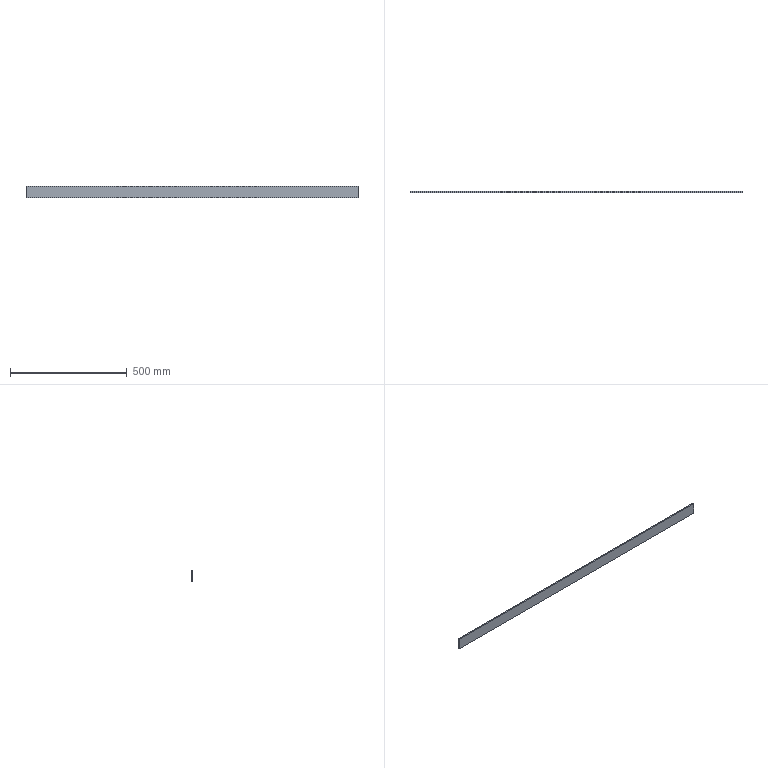Part | STEP file | Gripper baffle | 1 solid | 6 faces | box 1420 x 5 x 50 mm | volume 355000 mm3 | plane 6
STEP:
#1=CARTESIAN_POINT('',(710.,0.,25.));
#2=VERTEX_POINT('',#1);
#3=CARTESIAN_POINT('',(710.,0.,-25.));
#4=VERTEX_POINT('',#3);
#5=CARTESIAN_POINT('',(710.,0.,-25.));
#6=DIRECTION('',(0.,0.,-1.));
#7=VECTOR('',#6,1000.);
#8=LINE('',#5,#7);
#9=EDGE_CURVE('',#2,#4,#8,.T.);
#10=ORIENTED_EDGE('',*,*,#9,.T.);
#11=CARTESIAN_POINT('',(710.,5.,-25.));
#12=VERTEX_POINT('',#11);
#13=CARTESIAN_POINT('',(710.,5.,-25.));
#14=DIRECTION('',(0.,-1.,0.));
#15=VECTOR('',#14,1000.);
#16=LINE('',#13,#15);
#17=EDGE_CURVE('',#12,#4,#16,.T.);
#18=ORIENTED_EDGE('',*,*,#17,.F.);
#19=CARTESIAN_POINT('',(710.,5.,25.));
#20=VERTEX_POINT('',#19);
#21=CARTESIAN_POINT('',(710.,5.,-25.));
#22=DIRECTION('',(0.,0.,-1.));
#23=VECTOR('',#22,1000.);
#24=LINE('',#21,#23);
#25=EDGE_CURVE('',#20,#12,#24,.T.);
#26=ORIENTED_EDGE('',*,*,#25,.F.);
#27=CARTESIAN_POINT('',(710.,5.,25.));
#28=DIRECTION('',(0.,-1.,0.));
#29=VECTOR('',#28,1000.);
#30=LINE('',#27,#29);
#31=EDGE_CURVE('',#20,#2,#30,.T.);
#32=ORIENTED_EDGE('',*,*,#31,.T.);
#33=EDGE_LOOP('',(#10,#18,#26,#32));
#34=FACE_OUTER_BOUND('',#33,.T.);
#35=CARTESIAN_POINT('',(710.,5.,-25.));
#36=DIRECTION('',(-1.,0.,0.));
#37=DIRECTION('',(0.,0.,1.));
#38=AXIS2_PLACEMENT_3D('',#35,#36,#37);
#39=PLANE('',#38);
#40=ADVANCED_FACE('',(#34),#39,.F.);
#41=CARTESIAN_POINT('',(-710.,0.,-25.));
#42=VERTEX_POINT('',#41);
#43=CARTESIAN_POINT('',(-710.,0.,-25.));
#44=DIRECTION('',(-1.,0.,0.));
#45=VECTOR('',#44,1000.);
#46=LINE('',#43,#45);
#47=EDGE_CURVE('',#4,#42,#46,.T.);
#48=ORIENTED_EDGE('',*,*,#47,.T.);
#49=CARTESIAN_POINT('',(-710.,5.,-25.));
#50=VERTEX_POINT('',#49);
#51=CARTESIAN_POINT('',(-710.,5.,-25.));
#52=DIRECTION('',(0.,-1.,0.));
#53=VECTOR('',#52,1000.);
#54=LINE('',#51,#53);
#55=EDGE_CURVE('',#50,#42,#54,.T.);
#56=ORIENTED_EDGE('',*,*,#55,.F.);
#57=CARTESIAN_POINT('',(-710.,5.,-25.));
#58=DIRECTION('',(-1.,0.,0.));
#59=VECTOR('',#58,1000.);
#60=LINE('',#57,#59);
#61=EDGE_CURVE('',#12,#50,#60,.T.);
#62=ORIENTED_EDGE('',*,*,#61,.F.);
#63=ORIENTED_EDGE('',*,*,#17,.T.);
#64=EDGE_LOOP('',(#48,#56,#62,#63));
#65=FACE_OUTER_BOUND('',#64,.T.);
#66=CARTESIAN_POINT('',(-710.,5.,-25.));
#67=DIRECTION('',(0.,0.,1.));
#68=DIRECTION('',(1.,0.,0.));
#69=AXIS2_PLACEMENT_3D('',#66,#67,#68);
#70=PLANE('',#69);
#71=ADVANCED_FACE('',(#65),#70,.F.);
#72=CARTESIAN_POINT('',(-710.,0.,25.));
#73=VERTEX_POINT('',#72);
#74=CARTESIAN_POINT('',(-710.,0.,-25.));
#75=DIRECTION('',(0.,0.,1.));
#76=VECTOR('',#75,1000.);
#77=LINE('',#74,#76);
#78=EDGE_CURVE('',#42,#73,#77,.T.);
#79=ORIENTED_EDGE('',*,*,#78,.T.);
#80=CARTESIAN_POINT('',(-710.,5.,25.));
#81=VERTEX_POINT('',#80);
#82=CARTESIAN_POINT('',(-710.,5.,25.));
#83=DIRECTION('',(0.,-1.,0.));
#84=VECTOR('',#83,1000.);
#85=LINE('',#82,#84);
#86=EDGE_CURVE('',#81,#73,#85,.T.);
#87=ORIENTED_EDGE('',*,*,#86,.F.);
#88=CARTESIAN_POINT('',(-710.,5.,-25.));
#89=DIRECTION('',(0.,0.,1.));
#90=VECTOR('',#89,1000.);
#91=LINE('',#88,#90);
#92=EDGE_CURVE('',#50,#81,#91,.T.);
#93=ORIENTED_EDGE('',*,*,#92,.F.);
#94=ORIENTED_EDGE('',*,*,#55,.T.);
#95=EDGE_LOOP('',(#79,#87,#93,#94));
#96=FACE_OUTER_BOUND('',#95,.T.);
#97=CARTESIAN_POINT('',(-710.,5.,-25.));
#98=DIRECTION('',(1.,0.,0.));
#99=DIRECTION('',(0.,0.,-1.));
#100=AXIS2_PLACEMENT_3D('',#97,#98,#99);
#101=PLANE('',#100);
#102=ADVANCED_FACE('',(#96),#101,.F.);
#103=CARTESIAN_POINT('',(-710.,0.,25.));
#104=DIRECTION('',(1.,0.,0.));
#105=VECTOR('',#104,1000.);
#106=LINE('',#103,#105);
#107=EDGE_CURVE('',#73,#2,#106,.T.);
#108=ORIENTED_EDGE('',*,*,#107,.T.);
#109=ORIENTED_EDGE('',*,*,#31,.F.);
#110=CARTESIAN_POINT('',(-710.,5.,25.));
#111=DIRECTION('',(1.,0.,0.));
#112=VECTOR('',#111,1000.);
#113=LINE('',#110,#112);
#114=EDGE_CURVE('',#81,#20,#113,.T.);
#115=ORIENTED_EDGE('',*,*,#114,.F.);
#116=ORIENTED_EDGE('',*,*,#86,.T.);
#117=EDGE_LOOP('',(#108,#109,#115,#116));
#118=FACE_OUTER_BOUND('',#117,.T.);
#119=CARTESIAN_POINT('',(-710.,5.,25.));
#120=DIRECTION('',(0.,0.,-1.));
#121=DIRECTION('',(-1.,0.,0.));
#122=AXIS2_PLACEMENT_3D('',#119,#120,#121);
#123=PLANE('',#122);
#124=ADVANCED_FACE('',(#118),#123,.F.);
#125=ORIENTED_EDGE('',*,*,#25,.T.);
#126=ORIENTED_EDGE('',*,*,#61,.T.);
#127=ORIENTED_EDGE('',*,*,#92,.T.);
#128=ORIENTED_EDGE('',*,*,#114,.T.);
#129=EDGE_LOOP('',(#125,#126,#127,#128));
#130=FACE_OUTER_BOUND('',#129,.T.);
#131=CARTESIAN_POINT('',(0.,5.,0.));
#132=DIRECTION('',(0.,1.,0.));
#133=DIRECTION('',(0.,0.,1.));
#134=AXIS2_PLACEMENT_3D('',#131,#132,#133);
#135=PLANE('',#134);
#136=ADVANCED_FACE('',(#130),#135,.T.);
#137=ORIENTED_EDGE('',*,*,#9,.F.);
#138=ORIENTED_EDGE('',*,*,#107,.F.);
#139=ORIENTED_EDGE('',*,*,#78,.F.);
#140=ORIENTED_EDGE('',*,*,#47,.F.);
#141=EDGE_LOOP('',(#137,#138,#139,#140));
#142=FACE_OUTER_BOUND('',#141,.T.);
#143=CARTESIAN_POINT('',(0.,0.,0.));
#144=DIRECTION('',(0.,1.,0.));
#145=DIRECTION('',(0.,0.,1.));
#146=AXIS2_PLACEMENT_3D('',#143,#144,#145);
#147=PLANE('',#146);
#148=ADVANCED_FACE('',(#142),#147,.F.);
#149=CLOSED_SHELL('',(#40,#71,#102,#124,#136,#148));
#150=MANIFOLD_SOLID_BREP('',#149);
#151=CARTESIAN_POINT('',(0.,0.,0.));
#152=DIRECTION('',(0.,0.,1.));
#153=DIRECTION('',(1.,0.,0.));
#154=AXIS2_PLACEMENT_3D('',#151,#152,#153);
#155=(LENGTH_UNIT()NAMED_UNIT(*)SI_UNIT(.MILLI.,.METRE.));
#156=UNCERTAINTY_MEASURE_WITH_UNIT(LENGTH_MEASURE(0.00001),#155,'','');
#157=(NAMED_UNIT(*)PLANE_ANGLE_UNIT()SI_UNIT($,.RADIAN.));
#158=(NAMED_UNIT(*)SI_UNIT($,.STERADIAN.)SOLID_ANGLE_UNIT());
#159=(GEOMETRIC_REPRESENTATION_CONTEXT(3)GLOBAL_UNCERTAINTY_ASSIGNED_CONTEXT((#156))GLOBAL_UNIT_ASSIGNED_CONTEXT((#155,#157,#158))REPRESENTATION_CONTEXT('',''));
#160=ADVANCED_BREP_SHAPE_REPRESENTATION('',(#150,#154),#159);